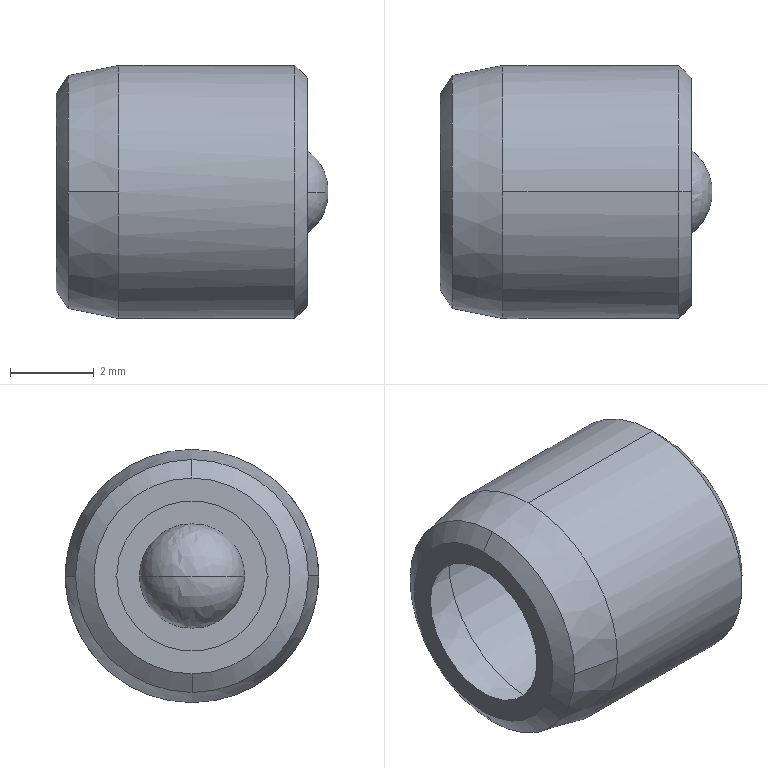Part | SolidWorks | features BaseBody 2 | 2 solids | 23 faces | box 6.5 x 6.04 x 6.04 mm | volume 46.835 mm3 | cone 12 | cylinder 6 | plane 3 | spline 2 | commonest cylinder face diameters 2 x2 5.44 x2 6.04 x2
STEP:
#1=CARTESIAN_POINT('',(5.7,0.,3.02));
#2=VERTEX_POINT('',#1);
#3=CARTESIAN_POINT('',(5.7,0.,-3.02));
#4=VERTEX_POINT('',#3);
#5=CARTESIAN_POINT('',(5.7,0.,0.));
#6=DIRECTION('',(-1.,0.,0.));
#7=DIRECTION('',(0.,0.,1.));
#8=AXIS2_PLACEMENT_3D('',#5,#6,#7);
#9=CIRCLE('',#8,3.02);
#10=EDGE_CURVE('',#2,#4,#9,.T.);
#11=ORIENTED_EDGE('',*,*,#10,.T.);
#12=CARTESIAN_POINT('',(1.5,0.,-3.02));
#13=VERTEX_POINT('',#12);
#14=CARTESIAN_POINT('',(0.,0.,-3.02));
#15=DIRECTION('',(-1.,0.,0.));
#16=VECTOR('',#15,1000.);
#17=LINE('',#14,#16);
#18=EDGE_CURVE('',#4,#13,#17,.T.);
#19=ORIENTED_EDGE('',*,*,#18,.T.);
#20=CARTESIAN_POINT('',(1.5,3.02,0.));
#21=VERTEX_POINT('',#20);
#22=CARTESIAN_POINT('',(1.5,0.,0.));
#23=DIRECTION('',(1.,0.,0.));
#24=DIRECTION('',(0.,0.,1.));
#25=AXIS2_PLACEMENT_3D('',#22,#23,#24);
#26=CIRCLE('',#25,3.02);
#27=EDGE_CURVE('',#13,#21,#26,.T.);
#28=ORIENTED_EDGE('',*,*,#27,.T.);
#29=CARTESIAN_POINT('',(1.5,0.,3.02));
#30=VERTEX_POINT('',#29);
#31=CARTESIAN_POINT('',(1.5,0.,0.));
#32=DIRECTION('',(1.,0.,0.));
#33=DIRECTION('',(0.,0.,1.));
#34=AXIS2_PLACEMENT_3D('',#31,#32,#33);
#35=CIRCLE('',#34,3.02);
#36=EDGE_CURVE('',#21,#30,#35,.T.);
#37=ORIENTED_EDGE('',*,*,#36,.T.);
#38=CARTESIAN_POINT('',(0.,0.,3.02));
#39=DIRECTION('',(-1.,0.,0.));
#40=VECTOR('',#39,1000.);
#41=LINE('',#38,#40);
#42=EDGE_CURVE('',#2,#30,#41,.T.);
#43=ORIENTED_EDGE('',*,*,#42,.F.);
#44=EDGE_LOOP('',(#11,#19,#28,#37,#43));
#45=FACE_OUTER_BOUND('',#44,.T.);
#46=CARTESIAN_POINT('',(0.,0.,0.));
#47=DIRECTION('',(-1.,0.,0.));
#48=DIRECTION('',(0.,0.,1.));
#49=AXIS2_PLACEMENT_3D('',#46,#47,#48);
#50=CYLINDRICAL_SURFACE('',#49,3.02);
#51=ADVANCED_FACE('',(#45),#50,.T.);
#52=CARTESIAN_POINT('',(0.2942,0.,2.779));
#53=VERTEX_POINT('',#52);
#54=CARTESIAN_POINT('',(0.2942,-2.779,0.));
#55=VERTEX_POINT('',#54);
#56=CARTESIAN_POINT('',(0.2942,0.,0.));
#57=DIRECTION('',(1.,0.,0.));
#58=DIRECTION('',(0.,0.,-1.));
#59=AXIS2_PLACEMENT_3D('',#56,#57,#58);
#60=CIRCLE('',#59,2.779);
#61=EDGE_CURVE('',#53,#55,#60,.T.);
#62=ORIENTED_EDGE('',*,*,#61,.T.);
#63=CARTESIAN_POINT('',(1.5,-3.02,0.));
#64=VERTEX_POINT('',#63);
#65=CARTESIAN_POINT('',(1.5,-3.02,0.));
#66=DIRECTION('',(0.9806,-0.1961,0.));
#67=VECTOR('',#66,1000.);
#68=LINE('',#65,#67);
#69=EDGE_CURVE('',#55,#64,#68,.T.);
#70=ORIENTED_EDGE('',*,*,#69,.T.);
#71=CARTESIAN_POINT('',(1.5,0.,0.));
#72=DIRECTION('',(1.,0.,0.));
#73=DIRECTION('',(0.,0.,1.));
#74=AXIS2_PLACEMENT_3D('',#71,#72,#73);
#75=CIRCLE('',#74,3.02);
#76=EDGE_CURVE('',#30,#64,#75,.T.);
#77=ORIENTED_EDGE('',*,*,#76,.F.);
#78=ORIENTED_EDGE('',*,*,#36,.F.);
#79=CARTESIAN_POINT('',(0.2942,2.779,0.));
#80=VERTEX_POINT('',#79);
#81=CARTESIAN_POINT('',(1.5,3.02,0.));
#82=DIRECTION('',(0.9806,0.1961,0.));
#83=VECTOR('',#82,1000.);
#84=LINE('',#81,#83);
#85=EDGE_CURVE('',#80,#21,#84,.T.);
#86=ORIENTED_EDGE('',*,*,#85,.F.);
#87=CARTESIAN_POINT('',(0.2942,0.,0.));
#88=DIRECTION('',(1.,0.,0.));
#89=DIRECTION('',(0.,0.,-1.));
#90=AXIS2_PLACEMENT_3D('',#87,#88,#89);
#91=CIRCLE('',#90,2.779);
#92=EDGE_CURVE('',#80,#53,#91,.T.);
#93=ORIENTED_EDGE('',*,*,#92,.T.);
#94=EDGE_LOOP('',(#62,#70,#77,#78,#86,#93));
#95=FACE_OUTER_BOUND('',#94,.T.);
#96=CARTESIAN_POINT('',(1.5,0.,0.));
#97=DIRECTION('',(1.,0.,0.));
#98=DIRECTION('',(0.,1.,0.));
#99=AXIS2_PLACEMENT_3D('',#96,#97,#98);
#100=CONICAL_SURFACE('',#99,3.02,0.1974);
#101=ADVANCED_FACE('',(#95),#100,.T.);
#102=CARTESIAN_POINT('',(6.,0.,2.72));
#103=VERTEX_POINT('',#102);
#104=CARTESIAN_POINT('',(6.,0.,-2.72));
#105=VERTEX_POINT('',#104);
#106=CARTESIAN_POINT('',(6.,0.,0.));
#107=DIRECTION('',(-1.,0.,0.));
#108=DIRECTION('',(0.,0.,1.));
#109=AXIS2_PLACEMENT_3D('',#106,#107,#108);
#110=CIRCLE('',#109,2.72);
#111=EDGE_CURVE('',#103,#105,#110,.T.);
#112=ORIENTED_EDGE('',*,*,#111,.T.);
#113=CARTESIAN_POINT('',(5.7,0.,-3.02));
#114=DIRECTION('',(-0.7071,0.,-0.7071));
#115=VECTOR('',#114,1000.);
#116=LINE('',#113,#115);
#117=EDGE_CURVE('',#105,#4,#116,.T.);
#118=ORIENTED_EDGE('',*,*,#117,.T.);
#119=ORIENTED_EDGE('',*,*,#10,.F.);
#120=CARTESIAN_POINT('',(5.7,0.,3.02));
#121=DIRECTION('',(-0.7071,0.,0.7071));
#122=VECTOR('',#121,1000.);
#123=LINE('',#120,#122);
#124=EDGE_CURVE('',#103,#2,#123,.T.);
#125=ORIENTED_EDGE('',*,*,#124,.F.);
#126=EDGE_LOOP('',(#112,#118,#119,#125));
#127=FACE_OUTER_BOUND('',#126,.T.);
#128=CARTESIAN_POINT('',(5.7,0.,0.));
#129=DIRECTION('',(-1.,0.,0.));
#130=DIRECTION('',(0.,0.,1.));
#131=AXIS2_PLACEMENT_3D('',#128,#129,#130);
#132=CONICAL_SURFACE('',#131,3.02,0.7854);
#133=ADVANCED_FACE('',(#127),#132,.T.);
#134=CARTESIAN_POINT('',(0.,0.,-2.338));
#135=VERTEX_POINT('',#134);
#136=CARTESIAN_POINT('',(0.,0.,2.338));
#137=VERTEX_POINT('',#136);
#138=CARTESIAN_POINT('',(0.,0.,0.));
#139=DIRECTION('',(1.,0.,0.));
#140=DIRECTION('',(0.,0.,-1.));
#141=AXIS2_PLACEMENT_3D('',#138,#139,#140);
#142=CIRCLE('',#141,2.338);
#143=EDGE_CURVE('',#135,#137,#142,.T.);
#144=ORIENTED_EDGE('',*,*,#143,.T.);
#145=CARTESIAN_POINT('',(0.2942,0.,2.779));
#146=DIRECTION('',(0.5547,0.,0.8321));
#147=VECTOR('',#146,1000.);
#148=LINE('',#145,#147);
#149=EDGE_CURVE('',#137,#53,#148,.T.);
#150=ORIENTED_EDGE('',*,*,#149,.T.);
#151=ORIENTED_EDGE('',*,*,#92,.F.);
#152=CARTESIAN_POINT('',(0.2942,0.,-2.779));
#153=VERTEX_POINT('',#152);
#154=CARTESIAN_POINT('',(0.2942,0.,0.));
#155=DIRECTION('',(1.,0.,0.));
#156=DIRECTION('',(0.,0.,-1.));
#157=AXIS2_PLACEMENT_3D('',#154,#155,#156);
#158=CIRCLE('',#157,2.779);
#159=EDGE_CURVE('',#153,#80,#158,.T.);
#160=ORIENTED_EDGE('',*,*,#159,.F.);
#161=CARTESIAN_POINT('',(0.2942,0.,-2.779));
#162=DIRECTION('',(0.5547,0.,-0.8321));
#163=VECTOR('',#162,1000.);
#164=LINE('',#161,#163);
#165=EDGE_CURVE('',#135,#153,#164,.T.);
#166=ORIENTED_EDGE('',*,*,#165,.F.);
#167=EDGE_LOOP('',(#144,#150,#151,#160,#166));
#168=FACE_OUTER_BOUND('',#167,.T.);
#169=CARTESIAN_POINT('',(0.2942,0.,0.));
#170=DIRECTION('',(1.,0.,0.));
#171=DIRECTION('',(0.,0.,-1.));
#172=AXIS2_PLACEMENT_3D('',#169,#170,#171);
#173=CONICAL_SURFACE('',#172,2.779,0.9828);
#174=ADVANCED_FACE('',(#168),#173,.T.);
#175=CARTESIAN_POINT('',(6.,0.,-1.));
#176=VERTEX_POINT('',#175);
#177=CARTESIAN_POINT('',(6.,0.,1.));
#178=VERTEX_POINT('',#177);
#179=CARTESIAN_POINT('',(6.,0.,0.));
#180=DIRECTION('',(-1.,0.,0.));
#181=DIRECTION('',(0.,0.,1.));
#182=AXIS2_PLACEMENT_3D('',#179,#180,#181);
#183=CIRCLE('',#182,1.);
#184=EDGE_CURVE('',#176,#178,#183,.T.);
#185=ORIENTED_EDGE('',*,*,#184,.F.);
#186=CARTESIAN_POINT('',(5.7,0.,-1.));
#187=VERTEX_POINT('',#186);
#188=CARTESIAN_POINT('',(15.7,0.,-1.));
#189=DIRECTION('',(-1.,0.,0.));
#190=VECTOR('',#189,1000.);
#191=LINE('',#188,#190);
#192=EDGE_CURVE('',#176,#187,#191,.T.);
#193=ORIENTED_EDGE('',*,*,#192,.T.);
#194=CARTESIAN_POINT('',(5.7,0.,1.));
#195=VERTEX_POINT('',#194);
#196=CARTESIAN_POINT('',(5.7,0.,0.));
#197=DIRECTION('',(1.,0.,0.));
#198=DIRECTION('',(0.,0.,1.));
#199=AXIS2_PLACEMENT_3D('',#196,#197,#198);
#200=CIRCLE('',#199,1.);
#201=EDGE_CURVE('',#195,#187,#200,.T.);
#202=ORIENTED_EDGE('',*,*,#201,.F.);
#203=CARTESIAN_POINT('',(15.7,0.,1.));
#204=DIRECTION('',(-1.,0.,0.));
#205=VECTOR('',#204,1000.);
#206=LINE('',#203,#205);
#207=EDGE_CURVE('',#178,#195,#206,.T.);
#208=ORIENTED_EDGE('',*,*,#207,.F.);
#209=EDGE_LOOP('',(#185,#193,#202,#208));
#210=FACE_OUTER_BOUND('',#209,.T.);
#211=CARTESIAN_POINT('',(15.7,0.,0.));
#212=DIRECTION('',(-1.,0.,0.));
#213=DIRECTION('',(0.,0.,1.));
#214=AXIS2_PLACEMENT_3D('',#211,#212,#213);
#215=CYLINDRICAL_SURFACE('',#214,1.);
#216=ADVANCED_FACE('',(#210),#215,.F.);
#217=CARTESIAN_POINT('',(0.,1.797,0.));
#218=VERTEX_POINT('',#217);
#219=CARTESIAN_POINT('',(0.,-1.797,0.));
#220=VERTEX_POINT('',#219);
#221=CARTESIAN_POINT('',(0.,0.,0.));
#222=DIRECTION('',(-1.,0.,0.));
#223=DIRECTION('',(0.,1.,0.));
#224=AXIS2_PLACEMENT_3D('',#221,#222,#223);
#225=CIRCLE('',#224,1.797);
#226=EDGE_CURVE('',#218,#220,#225,.T.);
#227=ORIENTED_EDGE('',*,*,#226,.T.);
#228=CARTESIAN_POINT('',(0.4749,-2.509,0.));
#229=VERTEX_POINT('',#228);
#230=CARTESIAN_POINT('',(0.4749,-2.509,0.));
#231=DIRECTION('',(0.5547,-0.8321,0.));
#232=VECTOR('',#231,1000.);
#233=LINE('',#230,#232);
#234=EDGE_CURVE('',#220,#229,#233,.T.);
#235=ORIENTED_EDGE('',*,*,#234,.T.);
#236=CARTESIAN_POINT('',(0.4749,0.,-2.509));
#237=VERTEX_POINT('',#236);
#238=CARTESIAN_POINT('',(0.4749,0.,0.));
#239=DIRECTION('',(-1.,0.,0.));
#240=DIRECTION('',(0.,0.,-1.));
#241=AXIS2_PLACEMENT_3D('',#238,#239,#240);
#242=CIRCLE('',#241,2.509);
#243=EDGE_CURVE('',#237,#229,#242,.T.);
#244=ORIENTED_EDGE('',*,*,#243,.F.);
#245=CARTESIAN_POINT('',(0.4749,2.509,0.));
#246=VERTEX_POINT('',#245);
#247=CARTESIAN_POINT('',(0.4749,0.,0.));
#248=DIRECTION('',(-1.,0.,0.));
#249=DIRECTION('',(0.,0.,-1.));
#250=AXIS2_PLACEMENT_3D('',#247,#248,#249);
#251=CIRCLE('',#250,2.509);
#252=EDGE_CURVE('',#246,#237,#251,.T.);
#253=ORIENTED_EDGE('',*,*,#252,.F.);
#254=CARTESIAN_POINT('',(0.4749,2.509,0.));
#255=DIRECTION('',(0.5547,0.8321,0.));
#256=VECTOR('',#255,1000.);
#257=LINE('',#254,#256);
#258=EDGE_CURVE('',#218,#246,#257,.T.);
#259=ORIENTED_EDGE('',*,*,#258,.F.);
#260=EDGE_LOOP('',(#227,#235,#244,#253,#259));
#261=FACE_OUTER_BOUND('',#260,.T.);
#262=CARTESIAN_POINT('',(0.4749,0.,0.));
#263=DIRECTION('',(1.,0.,0.));
#264=DIRECTION('',(0.,1.,0.));
#265=AXIS2_PLACEMENT_3D('',#262,#263,#264);
#266=CONICAL_SURFACE('',#265,2.509,0.9828);
#267=ADVANCED_FACE('',(#261),#266,.F.);
#268=ORIENTED_EDGE('',*,*,#243,.T.);
#269=CARTESIAN_POINT('',(0.4749,0.,2.509));
#270=VERTEX_POINT('',#269);
#271=CARTESIAN_POINT('',(0.4749,0.,0.));
#272=DIRECTION('',(-1.,0.,0.));
#273=DIRECTION('',(0.,0.,-1.));
#274=AXIS2_PLACEMENT_3D('',#271,#272,#273);
#275=CIRCLE('',#274,2.509);
#276=EDGE_CURVE('',#229,#270,#275,.T.);
#277=ORIENTED_EDGE('',*,*,#276,.T.);
#278=CARTESIAN_POINT('',(1.53,0.,2.72));
#279=VERTEX_POINT('',#278);
#280=CARTESIAN_POINT('',(1.53,0.,2.72));
#281=DIRECTION('',(0.9806,0.,0.1961));
#282=VECTOR('',#281,1000.);
#283=LINE('',#280,#282);
#284=EDGE_CURVE('',#270,#279,#283,.T.);
#285=ORIENTED_EDGE('',*,*,#284,.T.);
#286=CARTESIAN_POINT('',(1.53,0.,-2.72));
#287=VERTEX_POINT('',#286);
#288=CARTESIAN_POINT('',(1.53,0.,0.));
#289=DIRECTION('',(-1.,0.,0.));
#290=DIRECTION('',(0.,0.,-1.));
#291=AXIS2_PLACEMENT_3D('',#288,#289,#290);
#292=CIRCLE('',#291,2.72);
#293=EDGE_CURVE('',#287,#279,#292,.T.);
#294=ORIENTED_EDGE('',*,*,#293,.F.);
#295=CARTESIAN_POINT('',(1.53,0.,-2.72));
#296=DIRECTION('',(0.9806,0.,-0.1961));
#297=VECTOR('',#296,1000.);
#298=LINE('',#295,#297);
#299=EDGE_CURVE('',#237,#287,#298,.T.);
#300=ORIENTED_EDGE('',*,*,#299,.F.);
#301=EDGE_LOOP('',(#268,#277,#285,#294,#300));
#302=FACE_OUTER_BOUND('',#301,.T.);
#303=CARTESIAN_POINT('',(1.53,0.,0.));
#304=DIRECTION('',(1.,0.,0.));
#305=DIRECTION('',(0.,0.,-1.));
#306=AXIS2_PLACEMENT_3D('',#303,#304,#305);
#307=CONICAL_SURFACE('',#306,2.72,0.1974);
#308=ADVANCED_FACE('',(#302),#307,.F.);
#309=CARTESIAN_POINT('',(5.7,0.,2.596));
#310=VERTEX_POINT('',#309);
#311=CARTESIAN_POINT('',(5.7,0.,-2.596));
#312=VERTEX_POINT('',#311);
#313=CARTESIAN_POINT('',(5.7,0.,0.));
#314=DIRECTION('',(1.,0.,0.));
#315=DIRECTION('',(0.,0.,1.));
#316=AXIS2_PLACEMENT_3D('',#313,#314,#315);
#317=CIRCLE('',#316,2.596);
#318=EDGE_CURVE('',#310,#312,#317,.T.);
#319=ORIENTED_EDGE('',*,*,#318,.T.);
#320=CARTESIAN_POINT('',(5.576,0.,-2.72));
#321=VERTEX_POINT('',#320);
#322=CARTESIAN_POINT('',(5.576,0.,-2.72));
#323=DIRECTION('',(-0.7071,0.,-0.7071));
#324=VECTOR('',#323,1000.);
#325=LINE('',#322,#324);
#326=EDGE_CURVE('',#312,#321,#325,.T.);
#327=ORIENTED_EDGE('',*,*,#326,.T.);
#328=CARTESIAN_POINT('',(5.576,0.,2.72));
#329=VERTEX_POINT('',#328);
#330=CARTESIAN_POINT('',(5.576,0.,0.));
#331=DIRECTION('',(1.,0.,0.));
#332=DIRECTION('',(0.,0.,1.));
#333=AXIS2_PLACEMENT_3D('',#330,#331,#332);
#334=CIRCLE('',#333,2.72);
#335=EDGE_CURVE('',#329,#321,#334,.T.);
#336=ORIENTED_EDGE('',*,*,#335,.F.);
#337=CARTESIAN_POINT('',(5.576,0.,2.72));
#338=DIRECTION('',(-0.7071,0.,0.7071));
#339=VECTOR('',#338,1000.);
#340=LINE('',#337,#339);
#341=EDGE_CURVE('',#310,#329,#340,.T.);
#342=ORIENTED_EDGE('',*,*,#341,.F.);
#343=EDGE_LOOP('',(#319,#327,#336,#342));
#344=FACE_OUTER_BOUND('',#343,.T.);
#345=CARTESIAN_POINT('',(5.576,0.,0.));
#346=DIRECTION('',(-1.,0.,0.));
#347=DIRECTION('',(0.,0.,1.));
#348=AXIS2_PLACEMENT_3D('',#345,#346,#347);
#349=CONICAL_SURFACE('',#348,2.72,0.7854);
#350=ADVANCED_FACE('',(#344),#349,.F.);
#351=ORIENTED_EDGE('',*,*,#335,.T.);
#352=CARTESIAN_POINT('',(0.,0.,-2.72));
#353=DIRECTION('',(-1.,0.,0.));
#354=VECTOR('',#353,1000.);
#355=LINE('',#352,#354);
#356=EDGE_CURVE('',#321,#287,#355,.T.);
#357=ORIENTED_EDGE('',*,*,#356,.T.);
#358=ORIENTED_EDGE('',*,*,#293,.T.);
#359=CARTESIAN_POINT('',(0.,0.,2.72));
#360=DIRECTION('',(-1.,0.,0.));
#361=VECTOR('',#360,1000.);
#362=LINE('',#359,#361);
#363=EDGE_CURVE('',#329,#279,#362,.T.);
#364=ORIENTED_EDGE('',*,*,#363,.F.);
#365=EDGE_LOOP('',(#351,#357,#358,#364));
#366=FACE_OUTER_BOUND('',#365,.T.);
#367=CARTESIAN_POINT('',(0.,0.,0.));
#368=DIRECTION('',(-1.,0.,0.));
#369=DIRECTION('',(0.,0.,1.));
#370=AXIS2_PLACEMENT_3D('',#367,#368,#369);
#371=CYLINDRICAL_SURFACE('',#370,2.72);
#372=ADVANCED_FACE('',(#366),#371,.F.);
#373=ORIENTED_EDGE('',*,*,#18,.F.);
#374=CARTESIAN_POINT('',(5.7,0.,0.));
#375=DIRECTION('',(-1.,0.,0.));
#376=DIRECTION('',(0.,0.,1.));
#377=AXIS2_PLACEMENT_3D('',#374,#375,#376);
#378=CIRCLE('',#377,3.02);
#379=EDGE_CURVE('',#4,#2,#378,.T.);
#380=ORIENTED_EDGE('',*,*,#379,.T.);
#381=ORIENTED_EDGE('',*,*,#42,.T.);
#382=ORIENTED_EDGE('',*,*,#76,.T.);
#383=CARTESIAN_POINT('',(1.5,0.,0.));
#384=DIRECTION('',(1.,0.,0.));
#385=DIRECTION('',(0.,0.,1.));
#386=AXIS2_PLACEMENT_3D('',#383,#384,#385);
#387=CIRCLE('',#386,3.02);
#388=EDGE_CURVE('',#64,#13,#387,.T.);
#389=ORIENTED_EDGE('',*,*,#388,.T.);
#390=EDGE_LOOP('',(#373,#380,#381,#382,#389));
#391=FACE_OUTER_BOUND('',#390,.T.);
#392=CARTESIAN_POINT('',(0.,0.,0.));
#393=DIRECTION('',(-1.,0.,0.));
#394=DIRECTION('',(0.,0.,1.));
#395=AXIS2_PLACEMENT_3D('',#392,#393,#394);
#396=CYLINDRICAL_SURFACE('',#395,3.02);
#397=ADVANCED_FACE('',(#391),#396,.T.);
#398=ORIENTED_EDGE('',*,*,#69,.F.);
#399=CARTESIAN_POINT('',(0.2942,0.,0.));
#400=DIRECTION('',(1.,0.,0.));
#401=DIRECTION('',(0.,0.,-1.));
#402=AXIS2_PLACEMENT_3D('',#399,#400,#401);
#403=CIRCLE('',#402,2.779);
#404=EDGE_CURVE('',#55,#153,#403,.T.);
#405=ORIENTED_EDGE('',*,*,#404,.T.);
#406=ORIENTED_EDGE('',*,*,#159,.T.);
#407=ORIENTED_EDGE('',*,*,#85,.T.);
#408=ORIENTED_EDGE('',*,*,#27,.F.);
#409=ORIENTED_EDGE('',*,*,#388,.F.);
#410=EDGE_LOOP('',(#398,#405,#406,#407,#408,#409));
#411=FACE_OUTER_BOUND('',#410,.T.);
#412=CARTESIAN_POINT('',(1.5,0.,0.));
#413=DIRECTION('',(1.,0.,0.));
#414=DIRECTION('',(0.,1.,0.));
#415=AXIS2_PLACEMENT_3D('',#412,#413,#414);
#416=CONICAL_SURFACE('',#415,3.02,0.1974);
#417=ADVANCED_FACE('',(#411),#416,.T.);
#418=ORIENTED_EDGE('',*,*,#117,.F.);
#419=CARTESIAN_POINT('',(6.,0.,0.));
#420=DIRECTION('',(-1.,0.,0.));
#421=DIRECTION('',(0.,0.,1.));
#422=AXIS2_PLACEMENT_3D('',#419,#420,#421);
#423=CIRCLE('',#422,2.72);
#424=EDGE_CURVE('',#105,#103,#423,.T.);
#425=ORIENTED_EDGE('',*,*,#424,.T.);
#426=ORIENTED_EDGE('',*,*,#124,.T.);
#427=ORIENTED_EDGE('',*,*,#379,.F.);
#428=EDGE_LOOP('',(#418,#425,#426,#427));
#429=FACE_OUTER_BOUND('',#428,.T.);
#430=CARTESIAN_POINT('',(5.7,0.,0.));
#431=DIRECTION('',(-1.,0.,0.));
#432=DIRECTION('',(0.,0.,1.));
#433=AXIS2_PLACEMENT_3D('',#430,#431,#432);
#434=CONICAL_SURFACE('',#433,3.02,0.7854);
#435=ADVANCED_FACE('',(#429),#434,.T.);
#436=ORIENTED_EDGE('',*,*,#149,.F.);
#437=CARTESIAN_POINT('',(0.,0.,0.));
#438=DIRECTION('',(1.,0.,0.));
#439=DIRECTION('',(0.,0.,-1.));
#440=AXIS2_PLACEMENT_3D('',#437,#438,#439);
#441=CIRCLE('',#440,2.338);
#442=EDGE_CURVE('',#137,#135,#441,.T.);
#443=ORIENTED_EDGE('',*,*,#442,.T.);
#444=ORIENTED_EDGE('',*,*,#165,.T.);
#445=ORIENTED_EDGE('',*,*,#404,.F.);
#446=ORIENTED_EDGE('',*,*,#61,.F.);
#447=EDGE_LOOP('',(#436,#443,#444,#445,#446));
#448=FACE_OUTER_BOUND('',#447,.T.);
#449=CARTESIAN_POINT('',(0.2942,0.,0.));
#450=DIRECTION('',(1.,0.,0.));
#451=DIRECTION('',(0.,0.,-1.));
#452=AXIS2_PLACEMENT_3D('',#449,#450,#451);
#453=CONICAL_SURFACE('',#452,2.779,0.9828);
#454=ADVANCED_FACE('',(#448),#453,.T.);
#455=ORIENTED_EDGE('',*,*,#111,.F.);
#456=ORIENTED_EDGE('',*,*,#424,.F.);
#457=EDGE_LOOP('',(#455,#456));
#458=FACE_OUTER_BOUND('',#457,.T.);
#459=CARTESIAN_POINT('',(6.,0.,0.));
#460=DIRECTION('',(-1.,0.,0.));
#461=DIRECTION('',(0.,0.,1.));
#462=AXIS2_PLACEMENT_3D('',#459,#460,#461);
#463=CIRCLE('',#462,1.);
#464=EDGE_CURVE('',#178,#176,#463,.T.);
#465=ORIENTED_EDGE('',*,*,#464,.T.);
#466=ORIENTED_EDGE('',*,*,#184,.T.);
#467=EDGE_LOOP('',(#465,#466));
#468=FACE_BOUND('',#467,.T.);
#469=CARTESIAN_POINT('',(6.,0.,0.));
#470=DIRECTION('',(1.,0.,0.));
#471=DIRECTION('',(0.,0.,-1.));
#472=AXIS2_PLACEMENT_3D('',#469,#470,#471);
#473=PLANE('',#472);
#474=ADVANCED_FACE('',(#458,#468),#473,.T.);
#475=ORIENTED_EDGE('',*,*,#226,.F.);
#476=CARTESIAN_POINT('',(0.,0.,0.));
#477=DIRECTION('',(-1.,0.,0.));
#478=DIRECTION('',(0.,1.,0.));
#479=AXIS2_PLACEMENT_3D('',#476,#477,#478);
#480=CIRCLE('',#479,1.797);
#481=EDGE_CURVE('',#220,#218,#480,.T.);
#482=ORIENTED_EDGE('',*,*,#481,.F.);
#483=EDGE_LOOP('',(#475,#482));
#484=FACE_BOUND('',#483,.T.);
#485=ORIENTED_EDGE('',*,*,#143,.F.);
#486=ORIENTED_EDGE('',*,*,#442,.F.);
#487=EDGE_LOOP('',(#485,#486));
#488=FACE_OUTER_BOUND('',#487,.T.);
#489=CARTESIAN_POINT('',(0.,0.,0.));
#490=DIRECTION('',(1.,0.,0.));
#491=DIRECTION('',(0.,0.,-1.));
#492=AXIS2_PLACEMENT_3D('',#489,#490,#491);
#493=PLANE('',#492);
#494=ADVANCED_FACE('',(#484,#488),#493,.F.);
#495=ORIENTED_EDGE('',*,*,#192,.F.);
#496=ORIENTED_EDGE('',*,*,#464,.F.);
#497=ORIENTED_EDGE('',*,*,#207,.T.);
#498=CARTESIAN_POINT('',(5.7,0.,0.));
#499=DIRECTION('',(1.,0.,0.));
#500=DIRECTION('',(0.,0.,1.));
#501=AXIS2_PLACEMENT_3D('',#498,#499,#500);
#502=CIRCLE('',#501,1.);
#503=EDGE_CURVE('',#187,#195,#502,.T.);
#504=ORIENTED_EDGE('',*,*,#503,.F.);
#505=EDGE_LOOP('',(#495,#496,#497,#504));
#506=FACE_OUTER_BOUND('',#505,.T.);
#507=CARTESIAN_POINT('',(15.7,0.,0.));
#508=DIRECTION('',(-1.,0.,0.));
#509=DIRECTION('',(0.,0.,1.));
#510=AXIS2_PLACEMENT_3D('',#507,#508,#509);
#511=CYLINDRICAL_SURFACE('',#510,1.);
#512=ADVANCED_FACE('',(#506),#511,.F.);
#513=ORIENTED_EDGE('',*,*,#234,.F.);
#514=ORIENTED_EDGE('',*,*,#481,.T.);
#515=ORIENTED_EDGE('',*,*,#258,.T.);
#516=CARTESIAN_POINT('',(0.4749,0.,0.));
#517=DIRECTION('',(-1.,0.,0.));
#518=DIRECTION('',(0.,0.,-1.));
#519=AXIS2_PLACEMENT_3D('',#516,#517,#518);
#520=CIRCLE('',#519,2.509);
#521=EDGE_CURVE('',#270,#246,#520,.T.);
#522=ORIENTED_EDGE('',*,*,#521,.F.);
#523=ORIENTED_EDGE('',*,*,#276,.F.);
#524=EDGE_LOOP('',(#513,#514,#515,#522,#523));
#525=FACE_OUTER_BOUND('',#524,.T.);
#526=CARTESIAN_POINT('',(0.4749,0.,0.));
#527=DIRECTION('',(1.,0.,0.));
#528=DIRECTION('',(0.,1.,0.));
#529=AXIS2_PLACEMENT_3D('',#526,#527,#528);
#530=CONICAL_SURFACE('',#529,2.509,0.9828);
#531=ADVANCED_FACE('',(#525),#530,.F.);
#532=ORIENTED_EDGE('',*,*,#318,.F.);
#533=CARTESIAN_POINT('',(5.7,0.,0.));
#534=DIRECTION('',(1.,0.,0.));
#535=DIRECTION('',(0.,0.,1.));
#536=AXIS2_PLACEMENT_3D('',#533,#534,#535);
#537=CIRCLE('',#536,2.596);
#538=EDGE_CURVE('',#312,#310,#537,.T.);
#539=ORIENTED_EDGE('',*,*,#538,.F.);
#540=EDGE_LOOP('',(#532,#539));
#541=FACE_OUTER_BOUND('',#540,.T.);
#542=ORIENTED_EDGE('',*,*,#201,.T.);
#543=ORIENTED_EDGE('',*,*,#503,.T.);
#544=EDGE_LOOP('',(#542,#543));
#545=FACE_BOUND('',#544,.T.);
#546=CARTESIAN_POINT('',(5.7,0.,0.));
#547=DIRECTION('',(1.,0.,0.));
#548=DIRECTION('',(0.,0.,-1.));
#549=AXIS2_PLACEMENT_3D('',#546,#547,#548);
#550=PLANE('',#549);
#551=ADVANCED_FACE('',(#541,#545),#550,.F.);
#552=ORIENTED_EDGE('',*,*,#284,.F.);
#553=ORIENTED_EDGE('',*,*,#521,.T.);
#554=ORIENTED_EDGE('',*,*,#252,.T.);
#555=ORIENTED_EDGE('',*,*,#299,.T.);
#556=CARTESIAN_POINT('',(1.53,0.,0.));
#557=DIRECTION('',(-1.,0.,0.));
#558=DIRECTION('',(0.,0.,-1.));
#559=AXIS2_PLACEMENT_3D('',#556,#557,#558);
#560=CIRCLE('',#559,2.72);
#561=EDGE_CURVE('',#279,#287,#560,.T.);
#562=ORIENTED_EDGE('',*,*,#561,.F.);
#563=EDGE_LOOP('',(#552,#553,#554,#555,#562));
#564=FACE_OUTER_BOUND('',#563,.T.);
#565=CARTESIAN_POINT('',(1.53,0.,0.));
#566=DIRECTION('',(1.,0.,0.));
#567=DIRECTION('',(0.,0.,-1.));
#568=AXIS2_PLACEMENT_3D('',#565,#566,#567);
#569=CONICAL_SURFACE('',#568,2.72,0.1974);
#570=ADVANCED_FACE('',(#564),#569,.F.);
#571=ORIENTED_EDGE('',*,*,#326,.F.);
#572=ORIENTED_EDGE('',*,*,#538,.T.);
#573=ORIENTED_EDGE('',*,*,#341,.T.);
#574=CARTESIAN_POINT('',(5.576,0.,0.));
#575=DIRECTION('',(1.,0.,0.));
#576=DIRECTION('',(0.,0.,1.));
#577=AXIS2_PLACEMENT_3D('',#574,#575,#576);
#578=CIRCLE('',#577,2.72);
#579=EDGE_CURVE('',#321,#329,#578,.T.);
#580=ORIENTED_EDGE('',*,*,#579,.F.);
#581=EDGE_LOOP('',(#571,#572,#573,#580));
#582=FACE_OUTER_BOUND('',#581,.T.);
#583=CARTESIAN_POINT('',(5.576,0.,0.));
#584=DIRECTION('',(-1.,0.,0.));
#585=DIRECTION('',(0.,0.,1.));
#586=AXIS2_PLACEMENT_3D('',#583,#584,#585);
#587=CONICAL_SURFACE('',#586,2.72,0.7854);
#588=ADVANCED_FACE('',(#582),#587,.F.);
#589=ORIENTED_EDGE('',*,*,#356,.F.);
#590=ORIENTED_EDGE('',*,*,#579,.T.);
#591=ORIENTED_EDGE('',*,*,#363,.T.);
#592=ORIENTED_EDGE('',*,*,#561,.T.);
#593=EDGE_LOOP('',(#589,#590,#591,#592));
#594=FACE_OUTER_BOUND('',#593,.T.);
#595=CARTESIAN_POINT('',(0.,0.,0.));
#596=DIRECTION('',(-1.,0.,0.));
#597=DIRECTION('',(0.,0.,1.));
#598=AXIS2_PLACEMENT_3D('',#595,#596,#597);
#599=CYLINDRICAL_SURFACE('',#598,2.72);
#600=ADVANCED_FACE('',(#594),#599,.F.);
#601=CLOSED_SHELL('',(#51,#101,#133,#174,#216,#267,#308,#350,#372,#397,#417,#435,#454,#474,#494,#512,#531,#551,#570,#588,#600));
#602=MANIFOLD_SOLID_BREP('',#601);
#603=CARTESIAN_POINT('',(5.25,1.25,0.));
#604=VERTEX_POINT('',#603);
#605=CARTESIAN_POINT('',(5.25,-1.25,0.));
#606=VERTEX_POINT('',#605);
#607=CARTESIAN_POINT('',(5.25,0.,0.));
#608=DIRECTION('',(0.,0.,-1.));
#609=DIRECTION('',(0.,1.,0.));
#610=AXIS2_PLACEMENT_3D('',#607,#608,#609);
#611=CIRCLE('',#610,1.25);
#612=EDGE_CURVE('',#604,#606,#611,.T.);
#613=ORIENTED_EDGE('',*,*,#612,.F.);
#614=CARTESIAN_POINT('',(5.25,0.,0.));
#615=DIRECTION('',(0.,0.,1.));
#616=DIRECTION('',(0.,1.,0.));
#617=AXIS2_PLACEMENT_3D('',#614,#615,#616);
#618=CIRCLE('',#617,1.25);
#619=EDGE_CURVE('',#604,#606,#618,.T.);
#620=ORIENTED_EDGE('',*,*,#619,.T.);
#621=EDGE_LOOP('',(#613,#620));
#622=FACE_OUTER_BOUND('',#621,.T.);
#623=CARTESIAN_POINT('',(5.25,1.25,0.));
#624=CARTESIAN_POINT('',(5.25,1.25,0.));
#625=CARTESIAN_POINT('',(5.25,1.25,0.));
#626=CARTESIAN_POINT('',(5.25,1.25,0.));
#627=CARTESIAN_POINT('',(2.75,1.25,0.));
#628=CARTESIAN_POINT('',(2.75,1.25,5.));
#629=CARTESIAN_POINT('',(7.75,1.25,5.));
#630=CARTESIAN_POINT('',(7.75,1.25,0.));
#631=CARTESIAN_POINT('',(2.75,-1.25,0.));
#632=CARTESIAN_POINT('',(2.75,-1.25,5.));
#633=CARTESIAN_POINT('',(7.75,-1.25,5.));
#634=CARTESIAN_POINT('',(7.75,-1.25,0.));
#635=CARTESIAN_POINT('',(5.25,-1.25,0.));
#636=CARTESIAN_POINT('',(5.25,-1.25,0.));
#637=CARTESIAN_POINT('',(5.25,-1.25,0.));
#638=CARTESIAN_POINT('',(5.25,-1.25,0.));
#639=(BOUNDED_SURFACE()B_SPLINE_SURFACE(3,3,((#623,#624,#625,#626),(#627,#628,#629,#630),(#631,#632,#633,#634),(#635,#636,#637,#638)),.UNSPECIFIED.,.F.,.F.,.F.)B_SPLINE_SURFACE_WITH_KNOTS((4,4),(4,4),(0.,1.),(0.,1.),.UNSPECIFIED.)GEOMETRIC_REPRESENTATION_ITEM()RATIONAL_B_SPLINE_SURFACE(((1.,0.3333,0.3333,1.),(0.3333,0.1111,0.1111,0.3333),(0.3333,0.1111,0.1111,0.3333),(1.,0.3333,0.3333,1.)))REPRESENTATION_ITEM('')SURFACE());
#640=ADVANCED_FACE('',(#622),#639,.T.);
#641=ORIENTED_EDGE('',*,*,#619,.F.);
#642=ORIENTED_EDGE('',*,*,#612,.T.);
#643=EDGE_LOOP('',(#641,#642));
#644=FACE_OUTER_BOUND('',#643,.T.);
#645=CARTESIAN_POINT('',(5.25,1.25,0.));
#646=CARTESIAN_POINT('',(5.25,1.25,0.));
#647=CARTESIAN_POINT('',(5.25,1.25,0.));
#648=CARTESIAN_POINT('',(5.25,1.25,0.));
#649=CARTESIAN_POINT('',(7.75,1.25,0.));
#650=CARTESIAN_POINT('',(7.75,1.25,-5.));
#651=CARTESIAN_POINT('',(2.75,1.25,-5.));
#652=CARTESIAN_POINT('',(2.75,1.25,0.));
#653=CARTESIAN_POINT('',(7.75,-1.25,0.));
#654=CARTESIAN_POINT('',(7.75,-1.25,-5.));
#655=CARTESIAN_POINT('',(2.75,-1.25,-5.));
#656=CARTESIAN_POINT('',(2.75,-1.25,0.));
#657=CARTESIAN_POINT('',(5.25,-1.25,0.));
#658=CARTESIAN_POINT('',(5.25,-1.25,0.));
#659=CARTESIAN_POINT('',(5.25,-1.25,0.));
#660=CARTESIAN_POINT('',(5.25,-1.25,0.));
#661=(BOUNDED_SURFACE()B_SPLINE_SURFACE(3,3,((#645,#646,#647,#648),(#649,#650,#651,#652),(#653,#654,#655,#656),(#657,#658,#659,#660)),.UNSPECIFIED.,.F.,.F.,.F.)B_SPLINE_SURFACE_WITH_KNOTS((4,4),(4,4),(0.,1.),(0.,1.),.UNSPECIFIED.)GEOMETRIC_REPRESENTATION_ITEM()RATIONAL_B_SPLINE_SURFACE(((1.,0.3333,0.3333,1.),(0.3333,0.1111,0.1111,0.3333),(0.3333,0.1111,0.1111,0.3333),(1.,0.3333,0.3333,1.)))REPRESENTATION_ITEM('')SURFACE());
#662=ADVANCED_FACE('',(#644),#661,.T.);
#663=CLOSED_SHELL('',(#640,#662));
#664=MANIFOLD_SOLID_BREP('',#663);
#665=CARTESIAN_POINT('',(0.,0.,0.));
#666=DIRECTION('',(0.,0.,1.));
#667=DIRECTION('',(1.,0.,0.));
#668=AXIS2_PLACEMENT_3D('',#665,#666,#667);
#669=(LENGTH_UNIT()NAMED_UNIT(*)SI_UNIT(.MILLI.,.METRE.));
#670=UNCERTAINTY_MEASURE_WITH_UNIT(LENGTH_MEASURE(0.00001),#669,'','');
#671=(NAMED_UNIT(*)PLANE_ANGLE_UNIT()SI_UNIT($,.RADIAN.));
#672=(NAMED_UNIT(*)SI_UNIT($,.STERADIAN.)SOLID_ANGLE_UNIT());
#673=(GEOMETRIC_REPRESENTATION_CONTEXT(3)GLOBAL_UNCERTAINTY_ASSIGNED_CONTEXT((#670))GLOBAL_UNIT_ASSIGNED_CONTEXT((#669,#671,#672))REPRESENTATION_CONTEXT('',''));
#674=ADVANCED_BREP_SHAPE_REPRESENTATION('',(#602,#664,#668),#673);